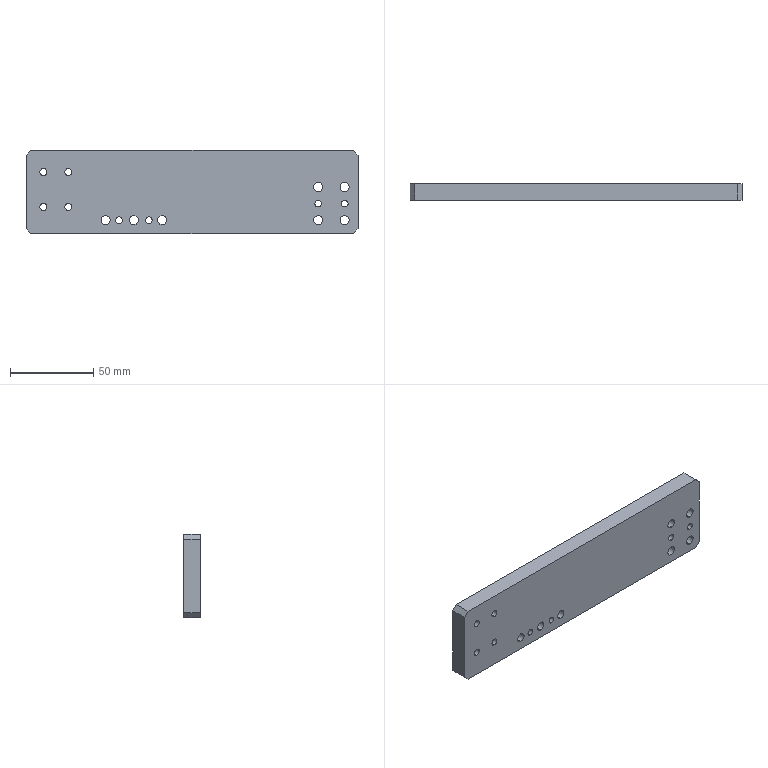Part | SolidWorks | features HoleWzd 5, Chamfer 1, Extrusion 1 | 1 solid | 40 faces | box 200 x 10 x 50 mm | volume 97100 mm3 | cylinder 30 | plane 10 | commonest cylinder face diameters 5.5 x14 4 x8 4.2 x8
STEP:
#1=CARTESIAN_POINT('',(-44.,10.,-19.));
#2=VERTEX_POINT('',#1);
#3=CARTESIAN_POINT('',(-44.,10.,-15.));
#4=VERTEX_POINT('',#3);
#5=CARTESIAN_POINT('',(-44.,10.,-17.));
#6=DIRECTION('',(0.,1.,0.));
#7=DIRECTION('',(0.,0.,1.));
#8=AXIS2_PLACEMENT_3D('',#5,#6,#7);
#9=CIRCLE('',#8,2.);
#10=EDGE_CURVE('',#2,#4,#9,.T.);
#11=ORIENTED_EDGE('',*,*,#10,.T.);
#12=CARTESIAN_POINT('',(-44.,0.,-15.));
#13=VERTEX_POINT('',#12);
#14=CARTESIAN_POINT('',(-44.,0.,-15.));
#15=DIRECTION('',(0.,-1.,0.));
#16=VECTOR('',#15,1000.);
#17=LINE('',#14,#16);
#18=EDGE_CURVE('',#4,#13,#17,.T.);
#19=ORIENTED_EDGE('',*,*,#18,.T.);
#20=CARTESIAN_POINT('',(-44.,0.,-19.));
#21=VERTEX_POINT('',#20);
#22=CARTESIAN_POINT('',(-44.,0.,-17.));
#23=DIRECTION('',(0.,-1.,0.));
#24=DIRECTION('',(0.,0.,-1.));
#25=AXIS2_PLACEMENT_3D('',#22,#23,#24);
#26=CIRCLE('',#25,2.);
#27=EDGE_CURVE('',#13,#21,#26,.T.);
#28=ORIENTED_EDGE('',*,*,#27,.T.);
#29=CARTESIAN_POINT('',(-44.,0.,-19.));
#30=DIRECTION('',(0.,-1.,0.));
#31=VECTOR('',#30,1000.);
#32=LINE('',#29,#31);
#33=EDGE_CURVE('',#2,#21,#32,.T.);
#34=ORIENTED_EDGE('',*,*,#33,.F.);
#35=EDGE_LOOP('',(#11,#19,#28,#34));
#36=FACE_OUTER_BOUND('',#35,.T.);
#37=CARTESIAN_POINT('',(-44.,0.,-17.));
#38=DIRECTION('',(0.,-1.,0.));
#39=DIRECTION('',(0.,0.,-1.));
#40=AXIS2_PLACEMENT_3D('',#37,#38,#39);
#41=CYLINDRICAL_SURFACE('',#40,2.);
#42=ADVANCED_FACE('',(#36),#41,.F.);
#43=CARTESIAN_POINT('',(-26.,10.,-19.));
#44=VERTEX_POINT('',#43);
#45=CARTESIAN_POINT('',(-26.,10.,-15.));
#46=VERTEX_POINT('',#45);
#47=CARTESIAN_POINT('',(-26.,10.,-17.));
#48=DIRECTION('',(0.,1.,0.));
#49=DIRECTION('',(0.,0.,1.));
#50=AXIS2_PLACEMENT_3D('',#47,#48,#49);
#51=CIRCLE('',#50,2.);
#52=EDGE_CURVE('',#44,#46,#51,.T.);
#53=ORIENTED_EDGE('',*,*,#52,.T.);
#54=CARTESIAN_POINT('',(-26.,0.,-15.));
#55=VERTEX_POINT('',#54);
#56=CARTESIAN_POINT('',(-26.,0.,-15.));
#57=DIRECTION('',(0.,-1.,0.));
#58=VECTOR('',#57,1000.);
#59=LINE('',#56,#58);
#60=EDGE_CURVE('',#46,#55,#59,.T.);
#61=ORIENTED_EDGE('',*,*,#60,.T.);
#62=CARTESIAN_POINT('',(-26.,0.,-19.));
#63=VERTEX_POINT('',#62);
#64=CARTESIAN_POINT('',(-26.,0.,-17.));
#65=DIRECTION('',(0.,-1.,0.));
#66=DIRECTION('',(0.,0.,-1.));
#67=AXIS2_PLACEMENT_3D('',#64,#65,#66);
#68=CIRCLE('',#67,2.);
#69=EDGE_CURVE('',#55,#63,#68,.T.);
#70=ORIENTED_EDGE('',*,*,#69,.T.);
#71=CARTESIAN_POINT('',(-26.,0.,-19.));
#72=DIRECTION('',(0.,-1.,0.));
#73=VECTOR('',#72,1000.);
#74=LINE('',#71,#73);
#75=EDGE_CURVE('',#44,#63,#74,.T.);
#76=ORIENTED_EDGE('',*,*,#75,.F.);
#77=EDGE_LOOP('',(#53,#61,#70,#76));
#78=FACE_OUTER_BOUND('',#77,.T.);
#79=CARTESIAN_POINT('',(-26.,0.,-17.));
#80=DIRECTION('',(0.,-1.,0.));
#81=DIRECTION('',(0.,0.,-1.));
#82=AXIS2_PLACEMENT_3D('',#79,#80,#81);
#83=CYLINDRICAL_SURFACE('',#82,2.);
#84=ADVANCED_FACE('',(#78),#83,.F.);
#85=CARTESIAN_POINT('',(-52.,10.,-19.75));
#86=VERTEX_POINT('',#85);
#87=CARTESIAN_POINT('',(-52.,10.,-14.25));
#88=VERTEX_POINT('',#87);
#89=CARTESIAN_POINT('',(-52.,10.,-17.));
#90=DIRECTION('',(0.,1.,0.));
#91=DIRECTION('',(0.,0.,1.));
#92=AXIS2_PLACEMENT_3D('',#89,#90,#91);
#93=CIRCLE('',#92,2.75);
#94=EDGE_CURVE('',#86,#88,#93,.T.);
#95=ORIENTED_EDGE('',*,*,#94,.T.);
#96=CARTESIAN_POINT('',(-52.,0.,-14.25));
#97=VERTEX_POINT('',#96);
#98=CARTESIAN_POINT('',(-52.,0.,-14.25));
#99=DIRECTION('',(0.,-1.,0.));
#100=VECTOR('',#99,1000.);
#101=LINE('',#98,#100);
#102=EDGE_CURVE('',#88,#97,#101,.T.);
#103=ORIENTED_EDGE('',*,*,#102,.T.);
#104=CARTESIAN_POINT('',(-52.,0.,-19.75));
#105=VERTEX_POINT('',#104);
#106=CARTESIAN_POINT('',(-52.,0.,-17.));
#107=DIRECTION('',(0.,-1.,0.));
#108=DIRECTION('',(0.,0.,-1.));
#109=AXIS2_PLACEMENT_3D('',#106,#107,#108);
#110=CIRCLE('',#109,2.75);
#111=EDGE_CURVE('',#97,#105,#110,.T.);
#112=ORIENTED_EDGE('',*,*,#111,.T.);
#113=CARTESIAN_POINT('',(-52.,0.,-19.75));
#114=DIRECTION('',(0.,-1.,0.));
#115=VECTOR('',#114,1000.);
#116=LINE('',#113,#115);
#117=EDGE_CURVE('',#86,#105,#116,.T.);
#118=ORIENTED_EDGE('',*,*,#117,.F.);
#119=EDGE_LOOP('',(#95,#103,#112,#118));
#120=FACE_OUTER_BOUND('',#119,.T.);
#121=CARTESIAN_POINT('',(-52.,0.,-17.));
#122=DIRECTION('',(0.,-1.,0.));
#123=DIRECTION('',(0.,0.,-1.));
#124=AXIS2_PLACEMENT_3D('',#121,#122,#123);
#125=CYLINDRICAL_SURFACE('',#124,2.75);
#126=ADVANCED_FACE('',(#120),#125,.F.);
#127=CARTESIAN_POINT('',(-35.,10.,-19.724));
#128=VERTEX_POINT('',#127);
#129=CARTESIAN_POINT('',(-35.,10.,-14.224));
#130=VERTEX_POINT('',#129);
#131=CARTESIAN_POINT('',(-35.,10.,-16.974));
#132=DIRECTION('',(0.,1.,0.));
#133=DIRECTION('',(0.,0.,1.));
#134=AXIS2_PLACEMENT_3D('',#131,#132,#133);
#135=CIRCLE('',#134,2.75);
#136=EDGE_CURVE('',#128,#130,#135,.T.);
#137=ORIENTED_EDGE('',*,*,#136,.T.);
#138=CARTESIAN_POINT('',(-35.,0.,-14.224));
#139=VERTEX_POINT('',#138);
#140=CARTESIAN_POINT('',(-35.,0.,-14.224));
#141=DIRECTION('',(0.,-1.,0.));
#142=VECTOR('',#141,1000.);
#143=LINE('',#140,#142);
#144=EDGE_CURVE('',#130,#139,#143,.T.);
#145=ORIENTED_EDGE('',*,*,#144,.T.);
#146=CARTESIAN_POINT('',(-35.,0.,-19.724));
#147=VERTEX_POINT('',#146);
#148=CARTESIAN_POINT('',(-35.,0.,-16.974));
#149=DIRECTION('',(0.,-1.,0.));
#150=DIRECTION('',(0.,0.,-1.));
#151=AXIS2_PLACEMENT_3D('',#148,#149,#150);
#152=CIRCLE('',#151,2.75);
#153=EDGE_CURVE('',#139,#147,#152,.T.);
#154=ORIENTED_EDGE('',*,*,#153,.T.);
#155=CARTESIAN_POINT('',(-35.,0.,-19.724));
#156=DIRECTION('',(0.,-1.,0.));
#157=VECTOR('',#156,1000.);
#158=LINE('',#155,#157);
#159=EDGE_CURVE('',#128,#147,#158,.T.);
#160=ORIENTED_EDGE('',*,*,#159,.F.);
#161=EDGE_LOOP('',(#137,#145,#154,#160));
#162=FACE_OUTER_BOUND('',#161,.T.);
#163=CARTESIAN_POINT('',(-35.,0.,-16.974));
#164=DIRECTION('',(0.,-1.,0.));
#165=DIRECTION('',(0.,0.,-1.));
#166=AXIS2_PLACEMENT_3D('',#163,#164,#165);
#167=CYLINDRICAL_SURFACE('',#166,2.75);
#168=ADVANCED_FACE('',(#162),#167,.F.);
#169=CARTESIAN_POINT('',(-18.,10.,-19.724));
#170=VERTEX_POINT('',#169);
#171=CARTESIAN_POINT('',(-18.,10.,-14.224));
#172=VERTEX_POINT('',#171);
#173=CARTESIAN_POINT('',(-18.,10.,-16.974));
#174=DIRECTION('',(0.,1.,0.));
#175=DIRECTION('',(0.,0.,1.));
#176=AXIS2_PLACEMENT_3D('',#173,#174,#175);
#177=CIRCLE('',#176,2.75);
#178=EDGE_CURVE('',#170,#172,#177,.T.);
#179=ORIENTED_EDGE('',*,*,#178,.T.);
#180=CARTESIAN_POINT('',(-18.,0.,-14.224));
#181=VERTEX_POINT('',#180);
#182=CARTESIAN_POINT('',(-18.,0.,-14.224));
#183=DIRECTION('',(0.,-1.,0.));
#184=VECTOR('',#183,1000.);
#185=LINE('',#182,#184);
#186=EDGE_CURVE('',#172,#181,#185,.T.);
#187=ORIENTED_EDGE('',*,*,#186,.T.);
#188=CARTESIAN_POINT('',(-18.,0.,-19.724));
#189=VERTEX_POINT('',#188);
#190=CARTESIAN_POINT('',(-18.,0.,-16.974));
#191=DIRECTION('',(0.,-1.,0.));
#192=DIRECTION('',(0.,0.,-1.));
#193=AXIS2_PLACEMENT_3D('',#190,#191,#192);
#194=CIRCLE('',#193,2.75);
#195=EDGE_CURVE('',#181,#189,#194,.T.);
#196=ORIENTED_EDGE('',*,*,#195,.T.);
#197=CARTESIAN_POINT('',(-18.,0.,-19.724));
#198=DIRECTION('',(0.,-1.,0.));
#199=VECTOR('',#198,1000.);
#200=LINE('',#197,#199);
#201=EDGE_CURVE('',#170,#189,#200,.T.);
#202=ORIENTED_EDGE('',*,*,#201,.F.);
#203=EDGE_LOOP('',(#179,#187,#196,#202));
#204=FACE_OUTER_BOUND('',#203,.T.);
#205=CARTESIAN_POINT('',(-18.,0.,-16.974));
#206=DIRECTION('',(0.,-1.,0.));
#207=DIRECTION('',(0.,0.,-1.));
#208=AXIS2_PLACEMENT_3D('',#205,#206,#207);
#209=CYLINDRICAL_SURFACE('',#208,2.75);
#210=ADVANCED_FACE('',(#204),#209,.F.);
#211=CARTESIAN_POINT('',(-89.5,0.,-11.1));
#212=VERTEX_POINT('',#211);
#213=CARTESIAN_POINT('',(-89.5,0.,-6.9));
#214=VERTEX_POINT('',#213);
#215=CARTESIAN_POINT('',(-89.5,0.,-9.));
#216=DIRECTION('',(0.,1.,0.));
#217=DIRECTION('',(0.,0.,1.));
#218=AXIS2_PLACEMENT_3D('',#215,#216,#217);
#219=CIRCLE('',#218,2.1);
#220=EDGE_CURVE('',#212,#214,#219,.T.);
#221=ORIENTED_EDGE('',*,*,#220,.F.);
#222=CARTESIAN_POINT('',(-89.5,10.,-11.1));
#223=VERTEX_POINT('',#222);
#224=CARTESIAN_POINT('',(-89.5,10.,-11.1));
#225=DIRECTION('',(0.,1.,0.));
#226=VECTOR('',#225,1000.);
#227=LINE('',#224,#226);
#228=EDGE_CURVE('',#212,#223,#227,.T.);
#229=ORIENTED_EDGE('',*,*,#228,.T.);
#230=CARTESIAN_POINT('',(-89.5,10.,-6.9));
#231=VERTEX_POINT('',#230);
#232=CARTESIAN_POINT('',(-89.5,10.,-9.));
#233=DIRECTION('',(0.,1.,0.));
#234=DIRECTION('',(0.,0.,1.));
#235=AXIS2_PLACEMENT_3D('',#232,#233,#234);
#236=CIRCLE('',#235,2.1);
#237=EDGE_CURVE('',#223,#231,#236,.T.);
#238=ORIENTED_EDGE('',*,*,#237,.T.);
#239=CARTESIAN_POINT('',(-89.5,10.,-6.9));
#240=DIRECTION('',(0.,1.,0.));
#241=VECTOR('',#240,1000.);
#242=LINE('',#239,#241);
#243=EDGE_CURVE('',#214,#231,#242,.T.);
#244=ORIENTED_EDGE('',*,*,#243,.F.);
#245=EDGE_LOOP('',(#221,#229,#238,#244));
#246=FACE_OUTER_BOUND('',#245,.T.);
#247=CARTESIAN_POINT('',(-89.5,10.,-9.));
#248=DIRECTION('',(0.,1.,0.));
#249=DIRECTION('',(0.,0.,1.));
#250=AXIS2_PLACEMENT_3D('',#247,#248,#249);
#251=CYLINDRICAL_SURFACE('',#250,2.1);
#252=ADVANCED_FACE('',(#246),#251,.F.);
#253=CARTESIAN_POINT('',(-74.5,0.,-11.1));
#254=VERTEX_POINT('',#253);
#255=CARTESIAN_POINT('',(-74.5,0.,-6.9));
#256=VERTEX_POINT('',#255);
#257=CARTESIAN_POINT('',(-74.5,0.,-9.));
#258=DIRECTION('',(0.,1.,0.));
#259=DIRECTION('',(0.,0.,1.));
#260=AXIS2_PLACEMENT_3D('',#257,#258,#259);
#261=CIRCLE('',#260,2.1);
#262=EDGE_CURVE('',#254,#256,#261,.T.);
#263=ORIENTED_EDGE('',*,*,#262,.F.);
#264=CARTESIAN_POINT('',(-74.5,10.,-11.1));
#265=VERTEX_POINT('',#264);
#266=CARTESIAN_POINT('',(-74.5,10.,-11.1));
#267=DIRECTION('',(0.,1.,0.));
#268=VECTOR('',#267,1000.);
#269=LINE('',#266,#268);
#270=EDGE_CURVE('',#254,#265,#269,.T.);
#271=ORIENTED_EDGE('',*,*,#270,.T.);
#272=CARTESIAN_POINT('',(-74.5,10.,-6.9));
#273=VERTEX_POINT('',#272);
#274=CARTESIAN_POINT('',(-74.5,10.,-9.));
#275=DIRECTION('',(0.,1.,0.));
#276=DIRECTION('',(0.,0.,1.));
#277=AXIS2_PLACEMENT_3D('',#274,#275,#276);
#278=CIRCLE('',#277,2.1);
#279=EDGE_CURVE('',#265,#273,#278,.T.);
#280=ORIENTED_EDGE('',*,*,#279,.T.);
#281=CARTESIAN_POINT('',(-74.5,10.,-6.9));
#282=DIRECTION('',(0.,1.,0.));
#283=VECTOR('',#282,1000.);
#284=LINE('',#281,#283);
#285=EDGE_CURVE('',#256,#273,#284,.T.);
#286=ORIENTED_EDGE('',*,*,#285,.F.);
#287=EDGE_LOOP('',(#263,#271,#280,#286));
#288=FACE_OUTER_BOUND('',#287,.T.);
#289=CARTESIAN_POINT('',(-74.5,10.,-9.));
#290=DIRECTION('',(0.,1.,0.));
#291=DIRECTION('',(0.,0.,1.));
#292=AXIS2_PLACEMENT_3D('',#289,#290,#291);
#293=CYLINDRICAL_SURFACE('',#292,2.1);
#294=ADVANCED_FACE('',(#288),#293,.F.);
#295=CARTESIAN_POINT('',(-89.5,0.,9.9));
#296=VERTEX_POINT('',#295);
#297=CARTESIAN_POINT('',(-89.5,0.,14.1));
#298=VERTEX_POINT('',#297);
#299=CARTESIAN_POINT('',(-89.5,0.,12.));
#300=DIRECTION('',(0.,1.,0.));
#301=DIRECTION('',(0.,0.,1.));
#302=AXIS2_PLACEMENT_3D('',#299,#300,#301);
#303=CIRCLE('',#302,2.1);
#304=EDGE_CURVE('',#296,#298,#303,.T.);
#305=ORIENTED_EDGE('',*,*,#304,.F.);
#306=CARTESIAN_POINT('',(-89.5,10.,9.9));
#307=VERTEX_POINT('',#306);
#308=CARTESIAN_POINT('',(-89.5,10.,9.9));
#309=DIRECTION('',(0.,1.,0.));
#310=VECTOR('',#309,1000.);
#311=LINE('',#308,#310);
#312=EDGE_CURVE('',#296,#307,#311,.T.);
#313=ORIENTED_EDGE('',*,*,#312,.T.);
#314=CARTESIAN_POINT('',(-89.5,10.,14.1));
#315=VERTEX_POINT('',#314);
#316=CARTESIAN_POINT('',(-89.5,10.,12.));
#317=DIRECTION('',(0.,1.,0.));
#318=DIRECTION('',(0.,0.,1.));
#319=AXIS2_PLACEMENT_3D('',#316,#317,#318);
#320=CIRCLE('',#319,2.1);
#321=EDGE_CURVE('',#307,#315,#320,.T.);
#322=ORIENTED_EDGE('',*,*,#321,.T.);
#323=CARTESIAN_POINT('',(-89.5,10.,14.1));
#324=DIRECTION('',(0.,1.,0.));
#325=VECTOR('',#324,1000.);
#326=LINE('',#323,#325);
#327=EDGE_CURVE('',#298,#315,#326,.T.);
#328=ORIENTED_EDGE('',*,*,#327,.F.);
#329=EDGE_LOOP('',(#305,#313,#322,#328));
#330=FACE_OUTER_BOUND('',#329,.T.);
#331=CARTESIAN_POINT('',(-89.5,10.,12.));
#332=DIRECTION('',(0.,1.,0.));
#333=DIRECTION('',(0.,0.,1.));
#334=AXIS2_PLACEMENT_3D('',#331,#332,#333);
#335=CYLINDRICAL_SURFACE('',#334,2.1);
#336=ADVANCED_FACE('',(#330),#335,.F.);
#337=CARTESIAN_POINT('',(-74.5,0.,9.9));
#338=VERTEX_POINT('',#337);
#339=CARTESIAN_POINT('',(-74.5,0.,14.1));
#340=VERTEX_POINT('',#339);
#341=CARTESIAN_POINT('',(-74.5,0.,12.));
#342=DIRECTION('',(0.,1.,0.));
#343=DIRECTION('',(0.,0.,1.));
#344=AXIS2_PLACEMENT_3D('',#341,#342,#343);
#345=CIRCLE('',#344,2.1);
#346=EDGE_CURVE('',#338,#340,#345,.T.);
#347=ORIENTED_EDGE('',*,*,#346,.F.);
#348=CARTESIAN_POINT('',(-74.5,10.,9.9));
#349=VERTEX_POINT('',#348);
#350=CARTESIAN_POINT('',(-74.5,10.,9.9));
#351=DIRECTION('',(0.,1.,0.));
#352=VECTOR('',#351,1000.);
#353=LINE('',#350,#352);
#354=EDGE_CURVE('',#338,#349,#353,.T.);
#355=ORIENTED_EDGE('',*,*,#354,.T.);
#356=CARTESIAN_POINT('',(-74.5,10.,14.1));
#357=VERTEX_POINT('',#356);
#358=CARTESIAN_POINT('',(-74.5,10.,12.));
#359=DIRECTION('',(0.,1.,0.));
#360=DIRECTION('',(0.,0.,1.));
#361=AXIS2_PLACEMENT_3D('',#358,#359,#360);
#362=CIRCLE('',#361,2.1);
#363=EDGE_CURVE('',#349,#357,#362,.T.);
#364=ORIENTED_EDGE('',*,*,#363,.T.);
#365=CARTESIAN_POINT('',(-74.5,10.,14.1));
#366=DIRECTION('',(0.,1.,0.));
#367=VECTOR('',#366,1000.);
#368=LINE('',#365,#367);
#369=EDGE_CURVE('',#340,#357,#368,.T.);
#370=ORIENTED_EDGE('',*,*,#369,.F.);
#371=EDGE_LOOP('',(#347,#355,#364,#370));
#372=FACE_OUTER_BOUND('',#371,.T.);
#373=CARTESIAN_POINT('',(-74.5,10.,12.));
#374=DIRECTION('',(0.,1.,0.));
#375=DIRECTION('',(0.,0.,1.));
#376=AXIS2_PLACEMENT_3D('',#373,#374,#375);
#377=CYLINDRICAL_SURFACE('',#376,2.1);
#378=ADVANCED_FACE('',(#372),#377,.F.);
#379=CARTESIAN_POINT('',(76.,0.,-9.));
#380=VERTEX_POINT('',#379);
#381=CARTESIAN_POINT('',(76.,0.,-5.));
#382=VERTEX_POINT('',#381);
#383=CARTESIAN_POINT('',(76.,0.,-7.));
#384=DIRECTION('',(0.,1.,0.));
#385=DIRECTION('',(0.,0.,1.));
#386=AXIS2_PLACEMENT_3D('',#383,#384,#385);
#387=CIRCLE('',#386,2.);
#388=EDGE_CURVE('',#380,#382,#387,.T.);
#389=ORIENTED_EDGE('',*,*,#388,.F.);
#390=CARTESIAN_POINT('',(76.,10.,-9.));
#391=VERTEX_POINT('',#390);
#392=CARTESIAN_POINT('',(76.,10.,-9.));
#393=DIRECTION('',(0.,1.,0.));
#394=VECTOR('',#393,1000.);
#395=LINE('',#392,#394);
#396=EDGE_CURVE('',#380,#391,#395,.T.);
#397=ORIENTED_EDGE('',*,*,#396,.T.);
#398=CARTESIAN_POINT('',(76.,10.,-5.));
#399=VERTEX_POINT('',#398);
#400=CARTESIAN_POINT('',(76.,10.,-7.));
#401=DIRECTION('',(0.,1.,0.));
#402=DIRECTION('',(0.,0.,1.));
#403=AXIS2_PLACEMENT_3D('',#400,#401,#402);
#404=CIRCLE('',#403,2.);
#405=EDGE_CURVE('',#391,#399,#404,.T.);
#406=ORIENTED_EDGE('',*,*,#405,.T.);
#407=CARTESIAN_POINT('',(76.,10.,-5.));
#408=DIRECTION('',(0.,1.,0.));
#409=VECTOR('',#408,1000.);
#410=LINE('',#407,#409);
#411=EDGE_CURVE('',#382,#399,#410,.T.);
#412=ORIENTED_EDGE('',*,*,#411,.F.);
#413=EDGE_LOOP('',(#389,#397,#406,#412));
#414=FACE_OUTER_BOUND('',#413,.T.);
#415=CARTESIAN_POINT('',(76.,10.,-7.));
#416=DIRECTION('',(0.,1.,0.));
#417=DIRECTION('',(0.,0.,1.));
#418=AXIS2_PLACEMENT_3D('',#415,#416,#417);
#419=CYLINDRICAL_SURFACE('',#418,2.);
#420=ADVANCED_FACE('',(#414),#419,.F.);
#421=CARTESIAN_POINT('',(92.,0.,-9.));
#422=VERTEX_POINT('',#421);
#423=CARTESIAN_POINT('',(92.,0.,-5.));
#424=VERTEX_POINT('',#423);
#425=CARTESIAN_POINT('',(92.,0.,-7.));
#426=DIRECTION('',(0.,1.,0.));
#427=DIRECTION('',(0.,0.,1.));
#428=AXIS2_PLACEMENT_3D('',#425,#426,#427);
#429=CIRCLE('',#428,2.);
#430=EDGE_CURVE('',#422,#424,#429,.T.);
#431=ORIENTED_EDGE('',*,*,#430,.F.);
#432=CARTESIAN_POINT('',(92.,10.,-9.));
#433=VERTEX_POINT('',#432);
#434=CARTESIAN_POINT('',(92.,10.,-9.));
#435=DIRECTION('',(0.,1.,0.));
#436=VECTOR('',#435,1000.);
#437=LINE('',#434,#436);
#438=EDGE_CURVE('',#422,#433,#437,.T.);
#439=ORIENTED_EDGE('',*,*,#438,.T.);
#440=CARTESIAN_POINT('',(92.,10.,-5.));
#441=VERTEX_POINT('',#440);
#442=CARTESIAN_POINT('',(92.,10.,-7.));
#443=DIRECTION('',(0.,1.,0.));
#444=DIRECTION('',(0.,0.,1.));
#445=AXIS2_PLACEMENT_3D('',#442,#443,#444);
#446=CIRCLE('',#445,2.);
#447=EDGE_CURVE('',#433,#441,#446,.T.);
#448=ORIENTED_EDGE('',*,*,#447,.T.);
#449=CARTESIAN_POINT('',(92.,10.,-5.));
#450=DIRECTION('',(0.,1.,0.));
#451=VECTOR('',#450,1000.);
#452=LINE('',#449,#451);
#453=EDGE_CURVE('',#424,#441,#452,.T.);
#454=ORIENTED_EDGE('',*,*,#453,.F.);
#455=EDGE_LOOP('',(#431,#439,#448,#454));
#456=FACE_OUTER_BOUND('',#455,.T.);
#457=CARTESIAN_POINT('',(92.,10.,-7.));
#458=DIRECTION('',(0.,1.,0.));
#459=DIRECTION('',(0.,0.,1.));
#460=AXIS2_PLACEMENT_3D('',#457,#458,#459);
#461=CYLINDRICAL_SURFACE('',#460,2.);
#462=ADVANCED_FACE('',(#456),#461,.F.);
#463=CARTESIAN_POINT('',(76.,0.,-19.75));
#464=VERTEX_POINT('',#463);
#465=CARTESIAN_POINT('',(76.,0.,-14.25));
#466=VERTEX_POINT('',#465);
#467=CARTESIAN_POINT('',(76.,0.,-17.));
#468=DIRECTION('',(0.,1.,0.));
#469=DIRECTION('',(0.,0.,1.));
#470=AXIS2_PLACEMENT_3D('',#467,#468,#469);
#471=CIRCLE('',#470,2.75);
#472=EDGE_CURVE('',#464,#466,#471,.T.);
#473=ORIENTED_EDGE('',*,*,#472,.F.);
#474=CARTESIAN_POINT('',(76.,10.,-19.75));
#475=VERTEX_POINT('',#474);
#476=CARTESIAN_POINT('',(76.,10.,-19.75));
#477=DIRECTION('',(0.,1.,0.));
#478=VECTOR('',#477,1000.);
#479=LINE('',#476,#478);
#480=EDGE_CURVE('',#464,#475,#479,.T.);
#481=ORIENTED_EDGE('',*,*,#480,.T.);
#482=CARTESIAN_POINT('',(76.,10.,-14.25));
#483=VERTEX_POINT('',#482);
#484=CARTESIAN_POINT('',(76.,10.,-17.));
#485=DIRECTION('',(0.,1.,0.));
#486=DIRECTION('',(0.,0.,1.));
#487=AXIS2_PLACEMENT_3D('',#484,#485,#486);
#488=CIRCLE('',#487,2.75);
#489=EDGE_CURVE('',#475,#483,#488,.T.);
#490=ORIENTED_EDGE('',*,*,#489,.T.);
#491=CARTESIAN_POINT('',(76.,10.,-14.25));
#492=DIRECTION('',(0.,1.,0.));
#493=VECTOR('',#492,1000.);
#494=LINE('',#491,#493);
#495=EDGE_CURVE('',#466,#483,#494,.T.);
#496=ORIENTED_EDGE('',*,*,#495,.F.);
#497=EDGE_LOOP('',(#473,#481,#490,#496));
#498=FACE_OUTER_BOUND('',#497,.T.);
#499=CARTESIAN_POINT('',(76.,10.,-17.));
#500=DIRECTION('',(0.,1.,0.));
#501=DIRECTION('',(0.,0.,1.));
#502=AXIS2_PLACEMENT_3D('',#499,#500,#501);
#503=CYLINDRICAL_SURFACE('',#502,2.75);
#504=ADVANCED_FACE('',(#498),#503,.F.);
#505=CARTESIAN_POINT('',(76.,0.,0.25));
#506=VERTEX_POINT('',#505);
#507=CARTESIAN_POINT('',(76.,0.,5.75));
#508=VERTEX_POINT('',#507);
#509=CARTESIAN_POINT('',(76.,0.,3.));
#510=DIRECTION('',(0.,1.,0.));
#511=DIRECTION('',(0.,0.,1.));
#512=AXIS2_PLACEMENT_3D('',#509,#510,#511);
#513=CIRCLE('',#512,2.75);
#514=EDGE_CURVE('',#506,#508,#513,.T.);
#515=ORIENTED_EDGE('',*,*,#514,.F.);
#516=CARTESIAN_POINT('',(76.,10.,0.25));
#517=VERTEX_POINT('',#516);
#518=CARTESIAN_POINT('',(76.,10.,0.25));
#519=DIRECTION('',(0.,1.,0.));
#520=VECTOR('',#519,1000.);
#521=LINE('',#518,#520);
#522=EDGE_CURVE('',#506,#517,#521,.T.);
#523=ORIENTED_EDGE('',*,*,#522,.T.);
#524=CARTESIAN_POINT('',(76.,10.,5.75));
#525=VERTEX_POINT('',#524);
#526=CARTESIAN_POINT('',(76.,10.,3.));
#527=DIRECTION('',(0.,1.,0.));
#528=DIRECTION('',(0.,0.,1.));
#529=AXIS2_PLACEMENT_3D('',#526,#527,#528);
#530=CIRCLE('',#529,2.75);
#531=EDGE_CURVE('',#517,#525,#530,.T.);
#532=ORIENTED_EDGE('',*,*,#531,.T.);
#533=CARTESIAN_POINT('',(76.,10.,5.75));
#534=DIRECTION('',(0.,1.,0.));
#535=VECTOR('',#534,1000.);
#536=LINE('',#533,#535);
#537=EDGE_CURVE('',#508,#525,#536,.T.);
#538=ORIENTED_EDGE('',*,*,#537,.F.);
#539=EDGE_LOOP('',(#515,#523,#532,#538));
#540=FACE_OUTER_BOUND('',#539,.T.);
#541=CARTESIAN_POINT('',(76.,10.,3.));
#542=DIRECTION('',(0.,1.,0.));
#543=DIRECTION('',(0.,0.,1.));
#544=AXIS2_PLACEMENT_3D('',#541,#542,#543);
#545=CYLINDRICAL_SURFACE('',#544,2.75);
#546=ADVANCED_FACE('',(#540),#545,.F.);
#547=CARTESIAN_POINT('',(92.,0.,0.25));
#548=VERTEX_POINT('',#547);
#549=CARTESIAN_POINT('',(92.,0.,5.75));
#550=VERTEX_POINT('',#549);
#551=CARTESIAN_POINT('',(92.,0.,3.));
#552=DIRECTION('',(0.,1.,0.));
#553=DIRECTION('',(0.,0.,1.));
#554=AXIS2_PLACEMENT_3D('',#551,#552,#553);
#555=CIRCLE('',#554,2.75);
#556=EDGE_CURVE('',#548,#550,#555,.T.);
#557=ORIENTED_EDGE('',*,*,#556,.F.);
#558=CARTESIAN_POINT('',(92.,10.,0.25));
#559=VERTEX_POINT('',#558);
#560=CARTESIAN_POINT('',(92.,10.,0.25));
#561=DIRECTION('',(0.,1.,0.));
#562=VECTOR('',#561,1000.);
#563=LINE('',#560,#562);
#564=EDGE_CURVE('',#548,#559,#563,.T.);
#565=ORIENTED_EDGE('',*,*,#564,.T.);
#566=CARTESIAN_POINT('',(92.,10.,5.75));
#567=VERTEX_POINT('',#566);
#568=CARTESIAN_POINT('',(92.,10.,3.));
#569=DIRECTION('',(0.,1.,0.));
#570=DIRECTION('',(0.,0.,1.));
#571=AXIS2_PLACEMENT_3D('',#568,#569,#570);
#572=CIRCLE('',#571,2.75);
#573=EDGE_CURVE('',#559,#567,#572,.T.);
#574=ORIENTED_EDGE('',*,*,#573,.T.);
#575=CARTESIAN_POINT('',(92.,10.,5.75));
#576=DIRECTION('',(0.,1.,0.));
#577=VECTOR('',#576,1000.);
#578=LINE('',#575,#577);
#579=EDGE_CURVE('',#550,#567,#578,.T.);
#580=ORIENTED_EDGE('',*,*,#579,.F.);
#581=EDGE_LOOP('',(#557,#565,#574,#580));
#582=FACE_OUTER_BOUND('',#581,.T.);
#583=CARTESIAN_POINT('',(92.,10.,3.));
#584=DIRECTION('',(0.,1.,0.));
#585=DIRECTION('',(0.,0.,1.));
#586=AXIS2_PLACEMENT_3D('',#583,#584,#585);
#587=CYLINDRICAL_SURFACE('',#586,2.75);
#588=ADVANCED_FACE('',(#582),#587,.F.);
#589=CARTESIAN_POINT('',(92.,0.,-19.75));
#590=VERTEX_POINT('',#589);
#591=CARTESIAN_POINT('',(92.,0.,-14.25));
#592=VERTEX_POINT('',#591);
#593=CARTESIAN_POINT('',(92.,0.,-17.));
#594=DIRECTION('',(0.,1.,0.));
#595=DIRECTION('',(0.,0.,1.));
#596=AXIS2_PLACEMENT_3D('',#593,#594,#595);
#597=CIRCLE('',#596,2.75);
#598=EDGE_CURVE('',#590,#592,#597,.T.);
#599=ORIENTED_EDGE('',*,*,#598,.F.);
#600=CARTESIAN_POINT('',(92.,10.,-19.75));
#601=VERTEX_POINT('',#600);
#602=CARTESIAN_POINT('',(92.,10.,-19.75));
#603=DIRECTION('',(0.,1.,0.));
#604=VECTOR('',#603,1000.);
#605=LINE('',#602,#604);
#606=EDGE_CURVE('',#590,#601,#605,.T.);
#607=ORIENTED_EDGE('',*,*,#606,.T.);
#608=CARTESIAN_POINT('',(92.,10.,-14.25));
#609=VERTEX_POINT('',#608);
#610=CARTESIAN_POINT('',(92.,10.,-17.));
#611=DIRECTION('',(0.,1.,0.));
#612=DIRECTION('',(0.,0.,1.));
#613=AXIS2_PLACEMENT_3D('',#610,#611,#612);
#614=CIRCLE('',#613,2.75);
#615=EDGE_CURVE('',#601,#609,#614,.T.);
#616=ORIENTED_EDGE('',*,*,#615,.T.);
#617=CARTESIAN_POINT('',(92.,10.,-14.25));
#618=DIRECTION('',(0.,1.,0.));
#619=VECTOR('',#618,1000.);
#620=LINE('',#617,#619);
#621=EDGE_CURVE('',#592,#609,#620,.T.);
#622=ORIENTED_EDGE('',*,*,#621,.F.);
#623=EDGE_LOOP('',(#599,#607,#616,#622));
#624=FACE_OUTER_BOUND('',#623,.T.);
#625=CARTESIAN_POINT('',(92.,10.,-17.));
#626=DIRECTION('',(0.,1.,0.));
#627=DIRECTION('',(0.,0.,1.));
#628=AXIS2_PLACEMENT_3D('',#625,#626,#627);
#629=CYLINDRICAL_SURFACE('',#628,2.75);
#630=ADVANCED_FACE('',(#624),#629,.F.);
#631=CARTESIAN_POINT('',(100.,10.,22.));
#632=VERTEX_POINT('',#631);
#633=CARTESIAN_POINT('',(100.,10.,-22.));
#634=VERTEX_POINT('',#633);
#635=CARTESIAN_POINT('',(100.,10.,-25.));
#636=DIRECTION('',(0.,0.,-1.));
#637=VECTOR('',#636,1000.);
#638=LINE('',#635,#637);
#639=EDGE_CURVE('',#632,#634,#638,.T.);
#640=ORIENTED_EDGE('',*,*,#639,.F.);
#641=CARTESIAN_POINT('',(100.,0.,22.));
#642=VERTEX_POINT('',#641);
#643=CARTESIAN_POINT('',(100.,10.,22.));
#644=DIRECTION('',(0.,-1.,0.));
#645=VECTOR('',#644,1000.);
#646=LINE('',#643,#645);
#647=EDGE_CURVE('',#632,#642,#646,.T.);
#648=ORIENTED_EDGE('',*,*,#647,.T.);
#649=CARTESIAN_POINT('',(100.,0.,-22.));
#650=VERTEX_POINT('',#649);
#651=CARTESIAN_POINT('',(100.,0.,-25.));
#652=DIRECTION('',(0.,0.,-1.));
#653=VECTOR('',#652,1000.);
#654=LINE('',#651,#653);
#655=EDGE_CURVE('',#642,#650,#654,.T.);
#656=ORIENTED_EDGE('',*,*,#655,.T.);
#657=CARTESIAN_POINT('',(100.,10.,-22.));
#658=DIRECTION('',(0.,1.,0.));
#659=VECTOR('',#658,1000.);
#660=LINE('',#657,#659);
#661=EDGE_CURVE('',#650,#634,#660,.T.);
#662=ORIENTED_EDGE('',*,*,#661,.T.);
#663=EDGE_LOOP('',(#640,#648,#656,#662));
#664=FACE_OUTER_BOUND('',#663,.T.);
#665=CARTESIAN_POINT('',(100.,10.,-25.));
#666=DIRECTION('',(-1.,0.,0.));
#667=DIRECTION('',(0.,0.,1.));
#668=AXIS2_PLACEMENT_3D('',#665,#666,#667);
#669=PLANE('',#668);
#670=ADVANCED_FACE('',(#664),#669,.F.);
#671=CARTESIAN_POINT('',(97.,10.,-25.));
#672=VERTEX_POINT('',#671);
#673=CARTESIAN_POINT('',(-97.,10.,-25.));
#674=VERTEX_POINT('',#673);
#675=CARTESIAN_POINT('',(-100.,10.,-25.));
#676=DIRECTION('',(-1.,0.,0.));
#677=VECTOR('',#676,1000.);
#678=LINE('',#675,#677);
#679=EDGE_CURVE('',#672,#674,#678,.T.);
#680=ORIENTED_EDGE('',*,*,#679,.F.);
#681=CARTESIAN_POINT('',(97.,0.,-25.));
#682=VERTEX_POINT('',#681);
#683=CARTESIAN_POINT('',(97.,10.,-25.));
#684=DIRECTION('',(0.,-1.,0.));
#685=VECTOR('',#684,1000.);
#686=LINE('',#683,#685);
#687=EDGE_CURVE('',#672,#682,#686,.T.);
#688=ORIENTED_EDGE('',*,*,#687,.T.);
#689=CARTESIAN_POINT('',(-97.,0.,-25.));
#690=VERTEX_POINT('',#689);
#691=CARTESIAN_POINT('',(-100.,0.,-25.));
#692=DIRECTION('',(-1.,0.,0.));
#693=VECTOR('',#692,1000.);
#694=LINE('',#691,#693);
#695=EDGE_CURVE('',#682,#690,#694,.T.);
#696=ORIENTED_EDGE('',*,*,#695,.T.);
#697=CARTESIAN_POINT('',(-97.,10.,-25.));
#698=DIRECTION('',(0.,1.,0.));
#699=VECTOR('',#698,1000.);
#700=LINE('',#697,#699);
#701=EDGE_CURVE('',#690,#674,#700,.T.);
#702=ORIENTED_EDGE('',*,*,#701,.T.);
#703=EDGE_LOOP('',(#680,#688,#696,#702));
#704=FACE_OUTER_BOUND('',#703,.T.);
#705=CARTESIAN_POINT('',(-100.,10.,-25.));
#706=DIRECTION('',(0.,0.,1.));
#707=DIRECTION('',(1.,0.,0.));
#708=AXIS2_PLACEMENT_3D('',#705,#706,#707);
#709=PLANE('',#708);
#710=ADVANCED_FACE('',(#704),#709,.F.);
#711=CARTESIAN_POINT('',(-100.,0.,-22.));
#712=VERTEX_POINT('',#711);
#713=CARTESIAN_POINT('',(-100.,0.,22.));
#714=VERTEX_POINT('',#713);
#715=CARTESIAN_POINT('',(-100.,0.,-25.));
#716=DIRECTION('',(0.,0.,1.));
#717=VECTOR('',#716,1000.);
#718=LINE('',#715,#717);
#719=EDGE_CURVE('',#712,#714,#718,.T.);
#720=ORIENTED_EDGE('',*,*,#719,.T.);
#721=CARTESIAN_POINT('',(-100.,10.,22.));
#722=VERTEX_POINT('',#721);
#723=CARTESIAN_POINT('',(-100.,10.,22.));
#724=DIRECTION('',(0.,1.,0.));
#725=VECTOR('',#724,1000.);
#726=LINE('',#723,#725);
#727=EDGE_CURVE('',#714,#722,#726,.T.);
#728=ORIENTED_EDGE('',*,*,#727,.T.);
#729=CARTESIAN_POINT('',(-100.,10.,-22.));
#730=VERTEX_POINT('',#729);
#731=CARTESIAN_POINT('',(-100.,10.,-25.));
#732=DIRECTION('',(0.,0.,1.));
#733=VECTOR('',#732,1000.);
#734=LINE('',#731,#733);
#735=EDGE_CURVE('',#730,#722,#734,.T.);
#736=ORIENTED_EDGE('',*,*,#735,.F.);
#737=CARTESIAN_POINT('',(-100.,10.,-22.));
#738=DIRECTION('',(0.,-1.,0.));
#739=VECTOR('',#738,1000.);
#740=LINE('',#737,#739);
#741=EDGE_CURVE('',#730,#712,#740,.T.);
#742=ORIENTED_EDGE('',*,*,#741,.T.);
#743=EDGE_LOOP('',(#720,#728,#736,#742));
#744=FACE_OUTER_BOUND('',#743,.T.);
#745=CARTESIAN_POINT('',(-100.,10.,-25.));
#746=DIRECTION('',(1.,0.,0.));
#747=DIRECTION('',(0.,0.,-1.));
#748=AXIS2_PLACEMENT_3D('',#745,#746,#747);
#749=PLANE('',#748);
#750=ADVANCED_FACE('',(#744),#749,.F.);
#751=CARTESIAN_POINT('',(-97.,0.,25.));
#752=VERTEX_POINT('',#751);
#753=CARTESIAN_POINT('',(97.,0.,25.));
#754=VERTEX_POINT('',#753);
#755=CARTESIAN_POINT('',(-100.,0.,25.));
#756=DIRECTION('',(1.,0.,0.));
#757=VECTOR('',#756,1000.);
#758=LINE('',#755,#757);
#759=EDGE_CURVE('',#752,#754,#758,.T.);
#760=ORIENTED_EDGE('',*,*,#759,.T.);
#761=CARTESIAN_POINT('',(97.,10.,25.));
#762=VERTEX_POINT('',#761);
#763=CARTESIAN_POINT('',(97.,10.,25.));
#764=DIRECTION('',(0.,1.,0.));
#765=VECTOR('',#764,1000.);
#766=LINE('',#763,#765);
#767=EDGE_CURVE('',#754,#762,#766,.T.);
#768=ORIENTED_EDGE('',*,*,#767,.T.);
#769=CARTESIAN_POINT('',(-97.,10.,25.));
#770=VERTEX_POINT('',#769);
#771=CARTESIAN_POINT('',(-100.,10.,25.));
#772=DIRECTION('',(1.,0.,0.));
#773=VECTOR('',#772,1000.);
#774=LINE('',#771,#773);
#775=EDGE_CURVE('',#770,#762,#774,.T.);
#776=ORIENTED_EDGE('',*,*,#775,.F.);
#777=CARTESIAN_POINT('',(-97.,10.,25.));
#778=DIRECTION('',(0.,-1.,0.));
#779=VECTOR('',#778,1000.);
#780=LINE('',#777,#779);
#781=EDGE_CURVE('',#770,#752,#780,.T.);
#782=ORIENTED_EDGE('',*,*,#781,.T.);
#783=EDGE_LOOP('',(#760,#768,#776,#782));
#784=FACE_OUTER_BOUND('',#783,.T.);
#785=CARTESIAN_POINT('',(-100.,10.,25.));
#786=DIRECTION('',(0.,0.,-1.));
#787=DIRECTION('',(-1.,0.,0.));
#788=AXIS2_PLACEMENT_3D('',#785,#786,#787);
#789=PLANE('',#788);
#790=ADVANCED_FACE('',(#784),#789,.F.);
#791=ORIENTED_EDGE('',*,*,#10,.F.);
#792=CARTESIAN_POINT('',(-44.,10.,-17.));
#793=DIRECTION('',(0.,1.,0.));
#794=DIRECTION('',(0.,0.,1.));
#795=AXIS2_PLACEMENT_3D('',#792,#793,#794);
#796=CIRCLE('',#795,2.);
#797=EDGE_CURVE('',#4,#2,#796,.T.);
#798=ORIENTED_EDGE('',*,*,#797,.F.);
#799=EDGE_LOOP('',(#791,#798));
#800=FACE_BOUND('',#799,.T.);
#801=ORIENTED_EDGE('',*,*,#52,.F.);
#802=CARTESIAN_POINT('',(-26.,10.,-17.));
#803=DIRECTION('',(0.,1.,0.));
#804=DIRECTION('',(0.,0.,1.));
#805=AXIS2_PLACEMENT_3D('',#802,#803,#804);
#806=CIRCLE('',#805,2.);
#807=EDGE_CURVE('',#46,#44,#806,.T.);
#808=ORIENTED_EDGE('',*,*,#807,.F.);
#809=EDGE_LOOP('',(#801,#808));
#810=FACE_BOUND('',#809,.T.);
#811=ORIENTED_EDGE('',*,*,#94,.F.);
#812=CARTESIAN_POINT('',(-52.,10.,-17.));
#813=DIRECTION('',(0.,1.,0.));
#814=DIRECTION('',(0.,0.,1.));
#815=AXIS2_PLACEMENT_3D('',#812,#813,#814);
#816=CIRCLE('',#815,2.75);
#817=EDGE_CURVE('',#88,#86,#816,.T.);
#818=ORIENTED_EDGE('',*,*,#817,.F.);
#819=EDGE_LOOP('',(#811,#818));
#820=FACE_BOUND('',#819,.T.);
#821=ORIENTED_EDGE('',*,*,#136,.F.);
#822=CARTESIAN_POINT('',(-35.,10.,-16.974));
#823=DIRECTION('',(0.,1.,0.));
#824=DIRECTION('',(0.,0.,1.));
#825=AXIS2_PLACEMENT_3D('',#822,#823,#824);
#826=CIRCLE('',#825,2.75);
#827=EDGE_CURVE('',#130,#128,#826,.T.);
#828=ORIENTED_EDGE('',*,*,#827,.F.);
#829=EDGE_LOOP('',(#821,#828));
#830=FACE_BOUND('',#829,.T.);
#831=ORIENTED_EDGE('',*,*,#178,.F.);
#832=CARTESIAN_POINT('',(-18.,10.,-16.974));
#833=DIRECTION('',(0.,1.,0.));
#834=DIRECTION('',(0.,0.,1.));
#835=AXIS2_PLACEMENT_3D('',#832,#833,#834);
#836=CIRCLE('',#835,2.75);
#837=EDGE_CURVE('',#172,#170,#836,.T.);
#838=ORIENTED_EDGE('',*,*,#837,.F.);
#839=EDGE_LOOP('',(#831,#838));
#840=FACE_BOUND('',#839,.T.);
#841=CARTESIAN_POINT('',(-89.5,10.,-9.));
#842=DIRECTION('',(0.,1.,0.));
#843=DIRECTION('',(0.,0.,1.));
#844=AXIS2_PLACEMENT_3D('',#841,#842,#843);
#845=CIRCLE('',#844,2.1);
#846=EDGE_CURVE('',#231,#223,#845,.T.);
#847=ORIENTED_EDGE('',*,*,#846,.F.);
#848=ORIENTED_EDGE('',*,*,#237,.F.);
#849=EDGE_LOOP('',(#847,#848));
#850=FACE_BOUND('',#849,.T.);
#851=CARTESIAN_POINT('',(-74.5,10.,-9.));
#852=DIRECTION('',(0.,1.,0.));
#853=DIRECTION('',(0.,0.,1.));
#854=AXIS2_PLACEMENT_3D('',#851,#852,#853);
#855=CIRCLE('',#854,2.1);
#856=EDGE_CURVE('',#273,#265,#855,.T.);
#857=ORIENTED_EDGE('',*,*,#856,.F.);
#858=ORIENTED_EDGE('',*,*,#279,.F.);
#859=EDGE_LOOP('',(#857,#858));
#860=FACE_BOUND('',#859,.T.);
#861=CARTESIAN_POINT('',(-89.5,10.,12.));
#862=DIRECTION('',(0.,1.,0.));
#863=DIRECTION('',(0.,0.,1.));
#864=AXIS2_PLACEMENT_3D('',#861,#862,#863);
#865=CIRCLE('',#864,2.1);
#866=EDGE_CURVE('',#315,#307,#865,.T.);
#867=ORIENTED_EDGE('',*,*,#866,.F.);
#868=ORIENTED_EDGE('',*,*,#321,.F.);
#869=EDGE_LOOP('',(#867,#868));
#870=FACE_BOUND('',#869,.T.);
#871=CARTESIAN_POINT('',(-74.5,10.,12.));
#872=DIRECTION('',(0.,1.,0.));
#873=DIRECTION('',(0.,0.,1.));
#874=AXIS2_PLACEMENT_3D('',#871,#872,#873);
#875=CIRCLE('',#874,2.1);
#876=EDGE_CURVE('',#357,#349,#875,.T.);
#877=ORIENTED_EDGE('',*,*,#876,.F.);
#878=ORIENTED_EDGE('',*,*,#363,.F.);
#879=EDGE_LOOP('',(#877,#878));
#880=FACE_BOUND('',#879,.T.);
#881=CARTESIAN_POINT('',(76.,10.,-7.));
#882=DIRECTION('',(0.,1.,0.));
#883=DIRECTION('',(0.,0.,1.));
#884=AXIS2_PLACEMENT_3D('',#881,#882,#883);
#885=CIRCLE('',#884,2.);
#886=EDGE_CURVE('',#399,#391,#885,.T.);
#887=ORIENTED_EDGE('',*,*,#886,.F.);
#888=ORIENTED_EDGE('',*,*,#405,.F.);
#889=EDGE_LOOP('',(#887,#888));
#890=FACE_BOUND('',#889,.T.);
#891=CARTESIAN_POINT('',(92.,10.,-7.));
#892=DIRECTION('',(0.,1.,0.));
#893=DIRECTION('',(0.,0.,1.));
#894=AXIS2_PLACEMENT_3D('',#891,#892,#893);
#895=CIRCLE('',#894,2.);
#896=EDGE_CURVE('',#441,#433,#895,.T.);
#897=ORIENTED_EDGE('',*,*,#896,.F.);
#898=ORIENTED_EDGE('',*,*,#447,.F.);
#899=EDGE_LOOP('',(#897,#898));
#900=FACE_BOUND('',#899,.T.);
#901=CARTESIAN_POINT('',(76.,10.,-17.));
#902=DIRECTION('',(0.,1.,0.));
#903=DIRECTION('',(0.,0.,1.));
#904=AXIS2_PLACEMENT_3D('',#901,#902,#903);
#905=CIRCLE('',#904,2.75);
#906=EDGE_CURVE('',#483,#475,#905,.T.);
#907=ORIENTED_EDGE('',*,*,#906,.F.);
#908=ORIENTED_EDGE('',*,*,#489,.F.);
#909=EDGE_LOOP('',(#907,#908));
#910=FACE_BOUND('',#909,.T.);
#911=CARTESIAN_POINT('',(76.,10.,3.));
#912=DIRECTION('',(0.,1.,0.));
#913=DIRECTION('',(0.,0.,1.));
#914=AXIS2_PLACEMENT_3D('',#911,#912,#913);
#915=CIRCLE('',#914,2.75);
#916=EDGE_CURVE('',#525,#517,#915,.T.);
#917=ORIENTED_EDGE('',*,*,#916,.F.);
#918=ORIENTED_EDGE('',*,*,#531,.F.);
#919=EDGE_LOOP('',(#917,#918));
#920=FACE_BOUND('',#919,.T.);
#921=CARTESIAN_POINT('',(92.,10.,3.));
#922=DIRECTION('',(0.,1.,0.));
#923=DIRECTION('',(0.,0.,1.));
#924=AXIS2_PLACEMENT_3D('',#921,#922,#923);
#925=CIRCLE('',#924,2.75);
#926=EDGE_CURVE('',#567,#559,#925,.T.);
#927=ORIENTED_EDGE('',*,*,#926,.F.);
#928=ORIENTED_EDGE('',*,*,#573,.F.);
#929=EDGE_LOOP('',(#927,#928));
#930=FACE_BOUND('',#929,.T.);
#931=CARTESIAN_POINT('',(92.,10.,-17.));
#932=DIRECTION('',(0.,1.,0.));
#933=DIRECTION('',(0.,0.,1.));
#934=AXIS2_PLACEMENT_3D('',#931,#932,#933);
#935=CIRCLE('',#934,2.75);
#936=EDGE_CURVE('',#609,#601,#935,.T.);
#937=ORIENTED_EDGE('',*,*,#936,.F.);
#938=ORIENTED_EDGE('',*,*,#615,.F.);
#939=EDGE_LOOP('',(#937,#938));
#940=FACE_BOUND('',#939,.T.);
#941=ORIENTED_EDGE('',*,*,#775,.T.);
#942=CARTESIAN_POINT('',(61.,10.,61.));
#943=DIRECTION('',(0.7071,0.,-0.7071));
#944=VECTOR('',#943,1000.);
#945=LINE('',#942,#944);
#946=EDGE_CURVE('',#762,#632,#945,.T.);
#947=ORIENTED_EDGE('',*,*,#946,.T.);
#948=ORIENTED_EDGE('',*,*,#639,.T.);
#949=CARTESIAN_POINT('',(61.,10.,-61.));
#950=DIRECTION('',(-0.7071,0.,-0.7071));
#951=VECTOR('',#950,1000.);
#952=LINE('',#949,#951);
#953=EDGE_CURVE('',#634,#672,#952,.T.);
#954=ORIENTED_EDGE('',*,*,#953,.T.);
#955=ORIENTED_EDGE('',*,*,#679,.T.);
#956=CARTESIAN_POINT('',(-61.,10.,-61.));
#957=DIRECTION('',(-0.7071,0.,0.7071));
#958=VECTOR('',#957,1000.);
#959=LINE('',#956,#958);
#960=EDGE_CURVE('',#674,#730,#959,.T.);
#961=ORIENTED_EDGE('',*,*,#960,.T.);
#962=ORIENTED_EDGE('',*,*,#735,.T.);
#963=CARTESIAN_POINT('',(-61.,10.,61.));
#964=DIRECTION('',(0.7071,0.,0.7071));
#965=VECTOR('',#964,1000.);
#966=LINE('',#963,#965);
#967=EDGE_CURVE('',#722,#770,#966,.T.);
#968=ORIENTED_EDGE('',*,*,#967,.T.);
#969=EDGE_LOOP('',(#941,#947,#948,#954,#955,#961,#962,#968));
#970=FACE_OUTER_BOUND('',#969,.T.);
#971=CARTESIAN_POINT('',(0.,10.,0.));
#972=DIRECTION('',(0.,1.,0.));
#973=DIRECTION('',(0.,0.,1.));
#974=AXIS2_PLACEMENT_3D('',#971,#972,#973);
#975=PLANE('',#974);
#976=ADVANCED_FACE('',(#800,#810,#820,#830,#840,#850,#860,#870,#880,#890,#900,#910,#920,#930,#940,#970),#975,.T.);
#977=CARTESIAN_POINT('',(-44.,0.,-17.));
#978=DIRECTION('',(0.,-1.,0.));
#979=DIRECTION('',(0.,0.,-1.));
#980=AXIS2_PLACEMENT_3D('',#977,#978,#979);
#981=CIRCLE('',#980,2.);
#982=EDGE_CURVE('',#21,#13,#981,.T.);
#983=ORIENTED_EDGE('',*,*,#982,.F.);
#984=ORIENTED_EDGE('',*,*,#27,.F.);
#985=EDGE_LOOP('',(#983,#984));
#986=FACE_BOUND('',#985,.T.);
#987=CARTESIAN_POINT('',(-26.,0.,-17.));
#988=DIRECTION('',(0.,-1.,0.));
#989=DIRECTION('',(0.,0.,-1.));
#990=AXIS2_PLACEMENT_3D('',#987,#988,#989);
#991=CIRCLE('',#990,2.);
#992=EDGE_CURVE('',#63,#55,#991,.T.);
#993=ORIENTED_EDGE('',*,*,#992,.F.);
#994=ORIENTED_EDGE('',*,*,#69,.F.);
#995=EDGE_LOOP('',(#993,#994));
#996=FACE_BOUND('',#995,.T.);
#997=CARTESIAN_POINT('',(-52.,0.,-17.));
#998=DIRECTION('',(0.,-1.,0.));
#999=DIRECTION('',(0.,0.,-1.));
#1000=AXIS2_PLACEMENT_3D('',#997,#998,#999);
#1001=CIRCLE('',#1000,2.75);
#1002=EDGE_CURVE('',#105,#97,#1001,.T.);
#1003=ORIENTED_EDGE('',*,*,#1002,.F.);
#1004=ORIENTED_EDGE('',*,*,#111,.F.);
#1005=EDGE_LOOP('',(#1003,#1004));
#1006=FACE_BOUND('',#1005,.T.);
#1007=CARTESIAN_POINT('',(-35.,0.,-16.974));
#1008=DIRECTION('',(0.,-1.,0.));
#1009=DIRECTION('',(0.,0.,-1.));
#1010=AXIS2_PLACEMENT_3D('',#1007,#1008,#1009);
#1011=CIRCLE('',#1010,2.75);
#1012=EDGE_CURVE('',#147,#139,#1011,.T.);
#1013=ORIENTED_EDGE('',*,*,#1012,.F.);
#1014=ORIENTED_EDGE('',*,*,#153,.F.);
#1015=EDGE_LOOP('',(#1013,#1014));
#1016=FACE_BOUND('',#1015,.T.);
#1017=CARTESIAN_POINT('',(-18.,0.,-16.974));
#1018=DIRECTION('',(0.,-1.,0.));
#1019=DIRECTION('',(0.,0.,-1.));
#1020=AXIS2_PLACEMENT_3D('',#1017,#1018,#1019);
#1021=CIRCLE('',#1020,2.75);
#1022=EDGE_CURVE('',#189,#181,#1021,.T.);
#1023=ORIENTED_EDGE('',*,*,#1022,.F.);
#1024=ORIENTED_EDGE('',*,*,#195,.F.);
#1025=EDGE_LOOP('',(#1023,#1024));
#1026=FACE_BOUND('',#1025,.T.);
#1027=CARTESIAN_POINT('',(-89.5,0.,-9.));
#1028=DIRECTION('',(0.,1.,0.));
#1029=DIRECTION('',(0.,0.,1.));
#1030=AXIS2_PLACEMENT_3D('',#1027,#1028,#1029);
#1031=CIRCLE('',#1030,2.1);
#1032=EDGE_CURVE('',#214,#212,#1031,.T.);
#1033=ORIENTED_EDGE('',*,*,#1032,.T.);
#1034=ORIENTED_EDGE('',*,*,#220,.T.);
#1035=EDGE_LOOP('',(#1033,#1034));
#1036=FACE_BOUND('',#1035,.T.);
#1037=CARTESIAN_POINT('',(-74.5,0.,-9.));
#1038=DIRECTION('',(0.,1.,0.));
#1039=DIRECTION('',(0.,0.,1.));
#1040=AXIS2_PLACEMENT_3D('',#1037,#1038,#1039);
#1041=CIRCLE('',#1040,2.1);
#1042=EDGE_CURVE('',#256,#254,#1041,.T.);
#1043=ORIENTED_EDGE('',*,*,#1042,.T.);
#1044=ORIENTED_EDGE('',*,*,#262,.T.);
#1045=EDGE_LOOP('',(#1043,#1044));
#1046=FACE_BOUND('',#1045,.T.);
#1047=CARTESIAN_POINT('',(-89.5,0.,12.));
#1048=DIRECTION('',(0.,1.,0.));
#1049=DIRECTION('',(0.,0.,1.));
#1050=AXIS2_PLACEMENT_3D('',#1047,#1048,#1049);
#1051=CIRCLE('',#1050,2.1);
#1052=EDGE_CURVE('',#298,#296,#1051,.T.);
#1053=ORIENTED_EDGE('',*,*,#1052,.T.);
#1054=ORIENTED_EDGE('',*,*,#304,.T.);
#1055=EDGE_LOOP('',(#1053,#1054));
#1056=FACE_BOUND('',#1055,.T.);
#1057=CARTESIAN_POINT('',(-74.5,0.,12.));
#1058=DIRECTION('',(0.,1.,0.));
#1059=DIRECTION('',(0.,0.,1.));
#1060=AXIS2_PLACEMENT_3D('',#1057,#1058,#1059);
#1061=CIRCLE('',#1060,2.1);
#1062=EDGE_CURVE('',#340,#338,#1061,.T.);
#1063=ORIENTED_EDGE('',*,*,#1062,.T.);
#1064=ORIENTED_EDGE('',*,*,#346,.T.);
#1065=EDGE_LOOP('',(#1063,#1064));
#1066=FACE_BOUND('',#1065,.T.);
#1067=CARTESIAN_POINT('',(76.,0.,-7.));
#1068=DIRECTION('',(0.,1.,0.));
#1069=DIRECTION('',(0.,0.,1.));
#1070=AXIS2_PLACEMENT_3D('',#1067,#1068,#1069);
#1071=CIRCLE('',#1070,2.);
#1072=EDGE_CURVE('',#382,#380,#1071,.T.);
#1073=ORIENTED_EDGE('',*,*,#1072,.T.);
#1074=ORIENTED_EDGE('',*,*,#388,.T.);
#1075=EDGE_LOOP('',(#1073,#1074));
#1076=FACE_BOUND('',#1075,.T.);
#1077=CARTESIAN_POINT('',(92.,0.,-7.));
#1078=DIRECTION('',(0.,1.,0.));
#1079=DIRECTION('',(0.,0.,1.));
#1080=AXIS2_PLACEMENT_3D('',#1077,#1078,#1079);
#1081=CIRCLE('',#1080,2.);
#1082=EDGE_CURVE('',#424,#422,#1081,.T.);
#1083=ORIENTED_EDGE('',*,*,#1082,.T.);
#1084=ORIENTED_EDGE('',*,*,#430,.T.);
#1085=EDGE_LOOP('',(#1083,#1084));
#1086=FACE_BOUND('',#1085,.T.);
#1087=CARTESIAN_POINT('',(76.,0.,-17.));
#1088=DIRECTION('',(0.,1.,0.));
#1089=DIRECTION('',(0.,0.,1.));
#1090=AXIS2_PLACEMENT_3D('',#1087,#1088,#1089);
#1091=CIRCLE('',#1090,2.75);
#1092=EDGE_CURVE('',#466,#464,#1091,.T.);
#1093=ORIENTED_EDGE('',*,*,#1092,.T.);
#1094=ORIENTED_EDGE('',*,*,#472,.T.);
#1095=EDGE_LOOP('',(#1093,#1094));
#1096=FACE_BOUND('',#1095,.T.);
#1097=CARTESIAN_POINT('',(76.,0.,3.));
#1098=DIRECTION('',(0.,1.,0.));
#1099=DIRECTION('',(0.,0.,1.));
#1100=AXIS2_PLACEMENT_3D('',#1097,#1098,#1099);
#1101=CIRCLE('',#1100,2.75);
#1102=EDGE_CURVE('',#508,#506,#1101,.T.);
#1103=ORIENTED_EDGE('',*,*,#1102,.T.);
#1104=ORIENTED_EDGE('',*,*,#514,.T.);
#1105=EDGE_LOOP('',(#1103,#1104));
#1106=FACE_BOUND('',#1105,.T.);
#1107=CARTESIAN_POINT('',(92.,0.,3.));
#1108=DIRECTION('',(0.,1.,0.));
#1109=DIRECTION('',(0.,0.,1.));
#1110=AXIS2_PLACEMENT_3D('',#1107,#1108,#1109);
#1111=CIRCLE('',#1110,2.75);
#1112=EDGE_CURVE('',#550,#548,#1111,.T.);
#1113=ORIENTED_EDGE('',*,*,#1112,.T.);
#1114=ORIENTED_EDGE('',*,*,#556,.T.);
#1115=EDGE_LOOP('',(#1113,#1114));
#1116=FACE_BOUND('',#1115,.T.);
#1117=CARTESIAN_POINT('',(92.,0.,-17.));
#1118=DIRECTION('',(0.,1.,0.));
#1119=DIRECTION('',(0.,0.,1.));
#1120=AXIS2_PLACEMENT_3D('',#1117,#1118,#1119);
#1121=CIRCLE('',#1120,2.75);
#1122=EDGE_CURVE('',#592,#590,#1121,.T.);
#1123=ORIENTED_EDGE('',*,*,#1122,.T.);
#1124=ORIENTED_EDGE('',*,*,#598,.T.);
#1125=EDGE_LOOP('',(#1123,#1124));
#1126=FACE_BOUND('',#1125,.T.);
#1127=ORIENTED_EDGE('',*,*,#655,.F.);
#1128=CARTESIAN_POINT('',(100.,0.,22.));
#1129=DIRECTION('',(-0.7071,0.,0.7071));
#1130=VECTOR('',#1129,1000.);
#1131=LINE('',#1128,#1130);
#1132=EDGE_CURVE('',#642,#754,#1131,.T.);
#1133=ORIENTED_EDGE('',*,*,#1132,.T.);
#1134=ORIENTED_EDGE('',*,*,#759,.F.);
#1135=CARTESIAN_POINT('',(-97.,0.,25.));
#1136=DIRECTION('',(-0.7071,0.,-0.7071));
#1137=VECTOR('',#1136,1000.);
#1138=LINE('',#1135,#1137);
#1139=EDGE_CURVE('',#752,#714,#1138,.T.);
#1140=ORIENTED_EDGE('',*,*,#1139,.T.);
#1141=ORIENTED_EDGE('',*,*,#719,.F.);
#1142=CARTESIAN_POINT('',(-100.,0.,-22.));
#1143=DIRECTION('',(0.7071,0.,-0.7071));
#1144=VECTOR('',#1143,1000.);
#1145=LINE('',#1142,#1144);
#1146=EDGE_CURVE('',#712,#690,#1145,.T.);
#1147=ORIENTED_EDGE('',*,*,#1146,.T.);
#1148=ORIENTED_EDGE('',*,*,#695,.F.);
#1149=CARTESIAN_POINT('',(97.,0.,-25.));
#1150=DIRECTION('',(0.7071,0.,0.7071));
#1151=VECTOR('',#1150,1000.);
#1152=LINE('',#1149,#1151);
#1153=EDGE_CURVE('',#682,#650,#1152,.T.);
#1154=ORIENTED_EDGE('',*,*,#1153,.T.);
#1155=EDGE_LOOP('',(#1127,#1133,#1134,#1140,#1141,#1147,#1148,#1154));
#1156=FACE_OUTER_BOUND('',#1155,.T.);
#1157=CARTESIAN_POINT('',(0.,0.,0.));
#1158=DIRECTION('',(0.,1.,0.));
#1159=DIRECTION('',(0.,0.,1.));
#1160=AXIS2_PLACEMENT_3D('',#1157,#1158,#1159);
#1161=PLANE('',#1160);
#1162=ADVANCED_FACE('',(#986,#996,#1006,#1016,#1026,#1036,#1046,#1056,#1066,#1076,#1086,#1096,#1106,#1116,#1126,#1156),#1161,.F.);
#1163=ORIENTED_EDGE('',*,*,#946,.F.);
#1164=ORIENTED_EDGE('',*,*,#767,.F.);
#1165=ORIENTED_EDGE('',*,*,#1132,.F.);
#1166=ORIENTED_EDGE('',*,*,#647,.F.);
#1167=EDGE_LOOP('',(#1163,#1164,#1165,#1166));
#1168=FACE_OUTER_BOUND('',#1167,.T.);
#1169=CARTESIAN_POINT('',(100.,10.,22.));
#1170=DIRECTION('',(-0.7071,0.,-0.7071));
#1171=DIRECTION('',(0.,-1.,0.));
#1172=AXIS2_PLACEMENT_3D('',#1169,#1170,#1171);
#1173=PLANE('',#1172);
#1174=ADVANCED_FACE('',(#1168),#1173,.F.);
#1175=ORIENTED_EDGE('',*,*,#953,.F.);
#1176=ORIENTED_EDGE('',*,*,#661,.F.);
#1177=ORIENTED_EDGE('',*,*,#1153,.F.);
#1178=ORIENTED_EDGE('',*,*,#687,.F.);
#1179=EDGE_LOOP('',(#1175,#1176,#1177,#1178));
#1180=FACE_OUTER_BOUND('',#1179,.T.);
#1181=CARTESIAN_POINT('',(97.,10.,-25.));
#1182=DIRECTION('',(-0.7071,0.,0.7071));
#1183=DIRECTION('',(0.,-1.,0.));
#1184=AXIS2_PLACEMENT_3D('',#1181,#1182,#1183);
#1185=PLANE('',#1184);
#1186=ADVANCED_FACE('',(#1180),#1185,.F.);
#1187=ORIENTED_EDGE('',*,*,#967,.F.);
#1188=ORIENTED_EDGE('',*,*,#727,.F.);
#1189=ORIENTED_EDGE('',*,*,#1139,.F.);
#1190=ORIENTED_EDGE('',*,*,#781,.F.);
#1191=EDGE_LOOP('',(#1187,#1188,#1189,#1190));
#1192=FACE_OUTER_BOUND('',#1191,.T.);
#1193=CARTESIAN_POINT('',(-97.,10.,25.));
#1194=DIRECTION('',(0.7071,0.,-0.7071));
#1195=DIRECTION('',(0.,-1.,0.));
#1196=AXIS2_PLACEMENT_3D('',#1193,#1194,#1195);
#1197=PLANE('',#1196);
#1198=ADVANCED_FACE('',(#1192),#1197,.F.);
#1199=ORIENTED_EDGE('',*,*,#960,.F.);
#1200=ORIENTED_EDGE('',*,*,#701,.F.);
#1201=ORIENTED_EDGE('',*,*,#1146,.F.);
#1202=ORIENTED_EDGE('',*,*,#741,.F.);
#1203=EDGE_LOOP('',(#1199,#1200,#1201,#1202));
#1204=FACE_OUTER_BOUND('',#1203,.T.);
#1205=CARTESIAN_POINT('',(-100.,10.,-22.));
#1206=DIRECTION('',(0.7071,0.,0.7071));
#1207=DIRECTION('',(0.,-1.,0.));
#1208=AXIS2_PLACEMENT_3D('',#1205,#1206,#1207);
#1209=PLANE('',#1208);
#1210=ADVANCED_FACE('',(#1204),#1209,.F.);
#1211=ORIENTED_EDGE('',*,*,#606,.F.);
#1212=ORIENTED_EDGE('',*,*,#1122,.F.);
#1213=ORIENTED_EDGE('',*,*,#621,.T.);
#1214=ORIENTED_EDGE('',*,*,#936,.T.);
#1215=EDGE_LOOP('',(#1211,#1212,#1213,#1214));
#1216=FACE_OUTER_BOUND('',#1215,.T.);
#1217=CARTESIAN_POINT('',(92.,10.,-17.));
#1218=DIRECTION('',(0.,1.,0.));
#1219=DIRECTION('',(0.,0.,1.));
#1220=AXIS2_PLACEMENT_3D('',#1217,#1218,#1219);
#1221=CYLINDRICAL_SURFACE('',#1220,2.75);
#1222=ADVANCED_FACE('',(#1216),#1221,.F.);
#1223=ORIENTED_EDGE('',*,*,#564,.F.);
#1224=ORIENTED_EDGE('',*,*,#1112,.F.);
#1225=ORIENTED_EDGE('',*,*,#579,.T.);
#1226=ORIENTED_EDGE('',*,*,#926,.T.);
#1227=EDGE_LOOP('',(#1223,#1224,#1225,#1226));
#1228=FACE_OUTER_BOUND('',#1227,.T.);
#1229=CARTESIAN_POINT('',(92.,10.,3.));
#1230=DIRECTION('',(0.,1.,0.));
#1231=DIRECTION('',(0.,0.,1.));
#1232=AXIS2_PLACEMENT_3D('',#1229,#1230,#1231);
#1233=CYLINDRICAL_SURFACE('',#1232,2.75);
#1234=ADVANCED_FACE('',(#1228),#1233,.F.);
#1235=ORIENTED_EDGE('',*,*,#522,.F.);
#1236=ORIENTED_EDGE('',*,*,#1102,.F.);
#1237=ORIENTED_EDGE('',*,*,#537,.T.);
#1238=ORIENTED_EDGE('',*,*,#916,.T.);
#1239=EDGE_LOOP('',(#1235,#1236,#1237,#1238));
#1240=FACE_OUTER_BOUND('',#1239,.T.);
#1241=CARTESIAN_POINT('',(76.,10.,3.));
#1242=DIRECTION('',(0.,1.,0.));
#1243=DIRECTION('',(0.,0.,1.));
#1244=AXIS2_PLACEMENT_3D('',#1241,#1242,#1243);
#1245=CYLINDRICAL_SURFACE('',#1244,2.75);
#1246=ADVANCED_FACE('',(#1240),#1245,.F.);
#1247=ORIENTED_EDGE('',*,*,#480,.F.);
#1248=ORIENTED_EDGE('',*,*,#1092,.F.);
#1249=ORIENTED_EDGE('',*,*,#495,.T.);
#1250=ORIENTED_EDGE('',*,*,#906,.T.);
#1251=EDGE_LOOP('',(#1247,#1248,#1249,#1250));
#1252=FACE_OUTER_BOUND('',#1251,.T.);
#1253=CARTESIAN_POINT('',(76.,10.,-17.));
#1254=DIRECTION('',(0.,1.,0.));
#1255=DIRECTION('',(0.,0.,1.));
#1256=AXIS2_PLACEMENT_3D('',#1253,#1254,#1255);
#1257=CYLINDRICAL_SURFACE('',#1256,2.75);
#1258=ADVANCED_FACE('',(#1252),#1257,.F.);
#1259=ORIENTED_EDGE('',*,*,#438,.F.);
#1260=ORIENTED_EDGE('',*,*,#1082,.F.);
#1261=ORIENTED_EDGE('',*,*,#453,.T.);
#1262=ORIENTED_EDGE('',*,*,#896,.T.);
#1263=EDGE_LOOP('',(#1259,#1260,#1261,#1262));
#1264=FACE_OUTER_BOUND('',#1263,.T.);
#1265=CARTESIAN_POINT('',(92.,10.,-7.));
#1266=DIRECTION('',(0.,1.,0.));
#1267=DIRECTION('',(0.,0.,1.));
#1268=AXIS2_PLACEMENT_3D('',#1265,#1266,#1267);
#1269=CYLINDRICAL_SURFACE('',#1268,2.);
#1270=ADVANCED_FACE('',(#1264),#1269,.F.);
#1271=ORIENTED_EDGE('',*,*,#396,.F.);
#1272=ORIENTED_EDGE('',*,*,#1072,.F.);
#1273=ORIENTED_EDGE('',*,*,#411,.T.);
#1274=ORIENTED_EDGE('',*,*,#886,.T.);
#1275=EDGE_LOOP('',(#1271,#1272,#1273,#1274));
#1276=FACE_OUTER_BOUND('',#1275,.T.);
#1277=CARTESIAN_POINT('',(76.,10.,-7.));
#1278=DIRECTION('',(0.,1.,0.));
#1279=DIRECTION('',(0.,0.,1.));
#1280=AXIS2_PLACEMENT_3D('',#1277,#1278,#1279);
#1281=CYLINDRICAL_SURFACE('',#1280,2.);
#1282=ADVANCED_FACE('',(#1276),#1281,.F.);
#1283=ORIENTED_EDGE('',*,*,#354,.F.);
#1284=ORIENTED_EDGE('',*,*,#1062,.F.);
#1285=ORIENTED_EDGE('',*,*,#369,.T.);
#1286=ORIENTED_EDGE('',*,*,#876,.T.);
#1287=EDGE_LOOP('',(#1283,#1284,#1285,#1286));
#1288=FACE_OUTER_BOUND('',#1287,.T.);
#1289=CARTESIAN_POINT('',(-74.5,10.,12.));
#1290=DIRECTION('',(0.,1.,0.));
#1291=DIRECTION('',(0.,0.,1.));
#1292=AXIS2_PLACEMENT_3D('',#1289,#1290,#1291);
#1293=CYLINDRICAL_SURFACE('',#1292,2.1);
#1294=ADVANCED_FACE('',(#1288),#1293,.F.);
#1295=ORIENTED_EDGE('',*,*,#312,.F.);
#1296=ORIENTED_EDGE('',*,*,#1052,.F.);
#1297=ORIENTED_EDGE('',*,*,#327,.T.);
#1298=ORIENTED_EDGE('',*,*,#866,.T.);
#1299=EDGE_LOOP('',(#1295,#1296,#1297,#1298));
#1300=FACE_OUTER_BOUND('',#1299,.T.);
#1301=CARTESIAN_POINT('',(-89.5,10.,12.));
#1302=DIRECTION('',(0.,1.,0.));
#1303=DIRECTION('',(0.,0.,1.));
#1304=AXIS2_PLACEMENT_3D('',#1301,#1302,#1303);
#1305=CYLINDRICAL_SURFACE('',#1304,2.1);
#1306=ADVANCED_FACE('',(#1300),#1305,.F.);
#1307=ORIENTED_EDGE('',*,*,#270,.F.);
#1308=ORIENTED_EDGE('',*,*,#1042,.F.);
#1309=ORIENTED_EDGE('',*,*,#285,.T.);
#1310=ORIENTED_EDGE('',*,*,#856,.T.);
#1311=EDGE_LOOP('',(#1307,#1308,#1309,#1310));
#1312=FACE_OUTER_BOUND('',#1311,.T.);
#1313=CARTESIAN_POINT('',(-74.5,10.,-9.));
#1314=DIRECTION('',(0.,1.,0.));
#1315=DIRECTION('',(0.,0.,1.));
#1316=AXIS2_PLACEMENT_3D('',#1313,#1314,#1315);
#1317=CYLINDRICAL_SURFACE('',#1316,2.1);
#1318=ADVANCED_FACE('',(#1312),#1317,.F.);
#1319=ORIENTED_EDGE('',*,*,#228,.F.);
#1320=ORIENTED_EDGE('',*,*,#1032,.F.);
#1321=ORIENTED_EDGE('',*,*,#243,.T.);
#1322=ORIENTED_EDGE('',*,*,#846,.T.);
#1323=EDGE_LOOP('',(#1319,#1320,#1321,#1322));
#1324=FACE_OUTER_BOUND('',#1323,.T.);
#1325=CARTESIAN_POINT('',(-89.5,10.,-9.));
#1326=DIRECTION('',(0.,1.,0.));
#1327=DIRECTION('',(0.,0.,1.));
#1328=AXIS2_PLACEMENT_3D('',#1325,#1326,#1327);
#1329=CYLINDRICAL_SURFACE('',#1328,2.1);
#1330=ADVANCED_FACE('',(#1324),#1329,.F.);
#1331=ORIENTED_EDGE('',*,*,#186,.F.);
#1332=ORIENTED_EDGE('',*,*,#837,.T.);
#1333=ORIENTED_EDGE('',*,*,#201,.T.);
#1334=ORIENTED_EDGE('',*,*,#1022,.T.);
#1335=EDGE_LOOP('',(#1331,#1332,#1333,#1334));
#1336=FACE_OUTER_BOUND('',#1335,.T.);
#1337=CARTESIAN_POINT('',(-18.,0.,-16.974));
#1338=DIRECTION('',(0.,-1.,0.));
#1339=DIRECTION('',(0.,0.,-1.));
#1340=AXIS2_PLACEMENT_3D('',#1337,#1338,#1339);
#1341=CYLINDRICAL_SURFACE('',#1340,2.75);
#1342=ADVANCED_FACE('',(#1336),#1341,.F.);
#1343=ORIENTED_EDGE('',*,*,#144,.F.);
#1344=ORIENTED_EDGE('',*,*,#827,.T.);
#1345=ORIENTED_EDGE('',*,*,#159,.T.);
#1346=ORIENTED_EDGE('',*,*,#1012,.T.);
#1347=EDGE_LOOP('',(#1343,#1344,#1345,#1346));
#1348=FACE_OUTER_BOUND('',#1347,.T.);
#1349=CARTESIAN_POINT('',(-35.,0.,-16.974));
#1350=DIRECTION('',(0.,-1.,0.));
#1351=DIRECTION('',(0.,0.,-1.));
#1352=AXIS2_PLACEMENT_3D('',#1349,#1350,#1351);
#1353=CYLINDRICAL_SURFACE('',#1352,2.75);
#1354=ADVANCED_FACE('',(#1348),#1353,.F.);
#1355=ORIENTED_EDGE('',*,*,#102,.F.);
#1356=ORIENTED_EDGE('',*,*,#817,.T.);
#1357=ORIENTED_EDGE('',*,*,#117,.T.);
#1358=ORIENTED_EDGE('',*,*,#1002,.T.);
#1359=EDGE_LOOP('',(#1355,#1356,#1357,#1358));
#1360=FACE_OUTER_BOUND('',#1359,.T.);
#1361=CARTESIAN_POINT('',(-52.,0.,-17.));
#1362=DIRECTION('',(0.,-1.,0.));
#1363=DIRECTION('',(0.,0.,-1.));
#1364=AXIS2_PLACEMENT_3D('',#1361,#1362,#1363);
#1365=CYLINDRICAL_SURFACE('',#1364,2.75);
#1366=ADVANCED_FACE('',(#1360),#1365,.F.);
#1367=ORIENTED_EDGE('',*,*,#60,.F.);
#1368=ORIENTED_EDGE('',*,*,#807,.T.);
#1369=ORIENTED_EDGE('',*,*,#75,.T.);
#1370=ORIENTED_EDGE('',*,*,#992,.T.);
#1371=EDGE_LOOP('',(#1367,#1368,#1369,#1370));
#1372=FACE_OUTER_BOUND('',#1371,.T.);
#1373=CARTESIAN_POINT('',(-26.,0.,-17.));
#1374=DIRECTION('',(0.,-1.,0.));
#1375=DIRECTION('',(0.,0.,-1.));
#1376=AXIS2_PLACEMENT_3D('',#1373,#1374,#1375);
#1377=CYLINDRICAL_SURFACE('',#1376,2.);
#1378=ADVANCED_FACE('',(#1372),#1377,.F.);
#1379=ORIENTED_EDGE('',*,*,#18,.F.);
#1380=ORIENTED_EDGE('',*,*,#797,.T.);
#1381=ORIENTED_EDGE('',*,*,#33,.T.);
#1382=ORIENTED_EDGE('',*,*,#982,.T.);
#1383=EDGE_LOOP('',(#1379,#1380,#1381,#1382));
#1384=FACE_OUTER_BOUND('',#1383,.T.);
#1385=CARTESIAN_POINT('',(-44.,0.,-17.));
#1386=DIRECTION('',(0.,-1.,0.));
#1387=DIRECTION('',(0.,0.,-1.));
#1388=AXIS2_PLACEMENT_3D('',#1385,#1386,#1387);
#1389=CYLINDRICAL_SURFACE('',#1388,2.);
#1390=ADVANCED_FACE('',(#1384),#1389,.F.);
#1391=CLOSED_SHELL('',(#42,#84,#126,#168,#210,#252,#294,#336,#378,#420,#462,#504,#546,#588,#630,#670,#710,#750,#790,#976,#1162,#1174,#1186,#1198,#1210,#1222,#1234,#1246,#1258,#1270,#1282,#1294,#1306,#1318,#1330,#1342,#1354,#1366,#1378,#1390));
#1392=MANIFOLD_SOLID_BREP('',#1391);
#1393=CARTESIAN_POINT('',(0.,0.,0.));
#1394=DIRECTION('',(0.,0.,1.));
#1395=DIRECTION('',(1.,0.,0.));
#1396=AXIS2_PLACEMENT_3D('',#1393,#1394,#1395);
#1397=(LENGTH_UNIT()NAMED_UNIT(*)SI_UNIT(.MILLI.,.METRE.));
#1398=UNCERTAINTY_MEASURE_WITH_UNIT(LENGTH_MEASURE(0.00001),#1397,'','');
#1399=(NAMED_UNIT(*)PLANE_ANGLE_UNIT()SI_UNIT($,.RADIAN.));
#1400=(NAMED_UNIT(*)SI_UNIT($,.STERADIAN.)SOLID_ANGLE_UNIT());
#1401=(GEOMETRIC_REPRESENTATION_CONTEXT(3)GLOBAL_UNCERTAINTY_ASSIGNED_CONTEXT((#1398))GLOBAL_UNIT_ASSIGNED_CONTEXT((#1397,#1399,#1400))REPRESENTATION_CONTEXT('',''));
#1402=ADVANCED_BREP_SHAPE_REPRESENTATION('',(#1392,#1396),#1401);